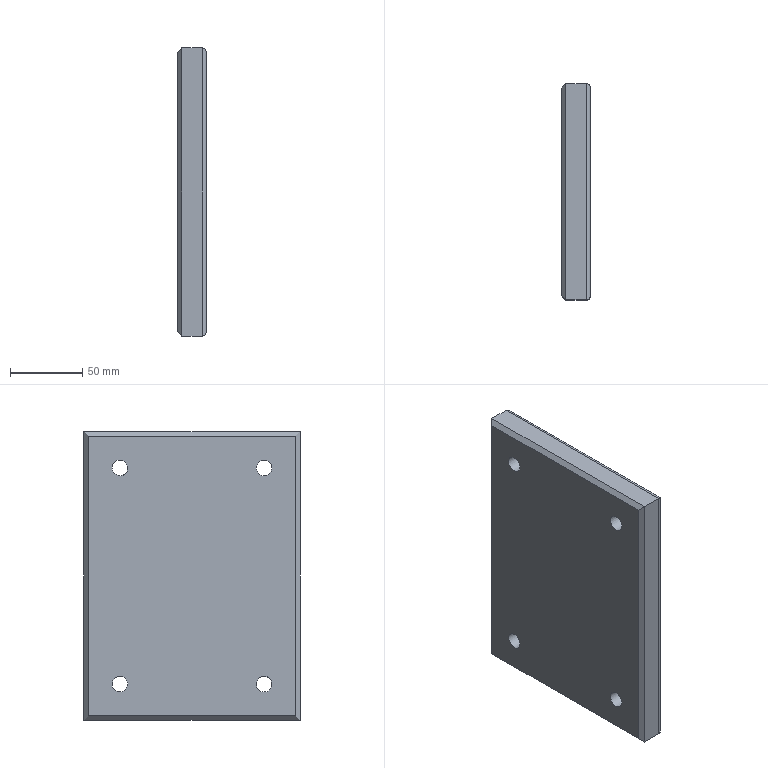Part | NX | features MAIN_BODY 2 | 1 solid | 30 faces | box 20 x 150 x 200 mm | volume 580501 mm3 | plane 14 | cylinder 12 | torus 4 | commonest cylinder face diameters 6 x4 11 x4 17.5 x4
STEP:
#1=CARTESIAN_POINT('',(910.,113.,-257.));
#2=VERTEX_POINT('',#1);
#3=CARTESIAN_POINT('',(910.,113.,-63.));
#4=VERTEX_POINT('',#3);
#5=CARTESIAN_POINT('',(910.,113.,-60.));
#6=DIRECTION('',(0.,0.,-1.));
#7=VECTOR('',#6,1000.);
#8=LINE('',#5,#7);
#9=EDGE_CURVE('',#2,#4,#8,.F.);
#10=ORIENTED_EDGE('',*,*,#9,.F.);
#11=CARTESIAN_POINT('',(910.,257.,-257.));
#12=VERTEX_POINT('',#11);
#13=CARTESIAN_POINT('',(910.,110.,-257.));
#14=DIRECTION('',(0.,1.,0.));
#15=VECTOR('',#14,1000.);
#16=LINE('',#13,#15);
#17=EDGE_CURVE('',#12,#2,#16,.F.);
#18=ORIENTED_EDGE('',*,*,#17,.F.);
#19=CARTESIAN_POINT('',(910.,257.,-63.));
#20=VERTEX_POINT('',#19);
#21=CARTESIAN_POINT('',(910.,257.,-260.));
#22=DIRECTION('',(0.,0.,1.));
#23=VECTOR('',#22,1000.);
#24=LINE('',#21,#23);
#25=EDGE_CURVE('',#20,#12,#24,.F.);
#26=ORIENTED_EDGE('',*,*,#25,.F.);
#27=CARTESIAN_POINT('',(910.,260.,-63.));
#28=DIRECTION('',(0.,-1.,0.));
#29=VECTOR('',#28,1000.);
#30=LINE('',#27,#29);
#31=EDGE_CURVE('',#4,#20,#30,.F.);
#32=ORIENTED_EDGE('',*,*,#31,.F.);
#33=EDGE_LOOP('',(#10,#18,#26,#32));
#34=FACE_BOUND('',#33,.T.);
#35=CARTESIAN_POINT('',(910.,135.,-96.75));
#36=VERTEX_POINT('',#35);
#37=CARTESIAN_POINT('',(910.,135.,-85.));
#38=DIRECTION('',(1.,0.,0.));
#39=DIRECTION('',(0.,0.,-1.));
#40=AXIS2_PLACEMENT_3D('',#37,#38,#39);
#41=CIRCLE('',#40,11.75);
#42=EDGE_CURVE('',#36,#36,#41,.T.);
#43=ORIENTED_EDGE('',*,*,#42,.F.);
#44=EDGE_LOOP('',(#43));
#45=FACE_BOUND('',#44,.T.);
#46=CARTESIAN_POINT('',(910.,235.,-96.75));
#47=VERTEX_POINT('',#46);
#48=CARTESIAN_POINT('',(910.,235.,-85.));
#49=DIRECTION('',(1.,0.,0.));
#50=DIRECTION('',(0.,0.,-1.));
#51=AXIS2_PLACEMENT_3D('',#48,#49,#50);
#52=CIRCLE('',#51,11.75);
#53=EDGE_CURVE('',#47,#47,#52,.T.);
#54=ORIENTED_EDGE('',*,*,#53,.F.);
#55=EDGE_LOOP('',(#54));
#56=FACE_BOUND('',#55,.T.);
#57=CARTESIAN_POINT('',(910.,235.,-246.75));
#58=VERTEX_POINT('',#57);
#59=CARTESIAN_POINT('',(910.,235.,-235.));
#60=DIRECTION('',(1.,0.,0.));
#61=DIRECTION('',(0.,0.,-1.));
#62=AXIS2_PLACEMENT_3D('',#59,#60,#61);
#63=CIRCLE('',#62,11.75);
#64=EDGE_CURVE('',#58,#58,#63,.T.);
#65=ORIENTED_EDGE('',*,*,#64,.F.);
#66=EDGE_LOOP('',(#65));
#67=FACE_BOUND('',#66,.T.);
#68=CARTESIAN_POINT('',(910.,135.,-246.75));
#69=VERTEX_POINT('',#68);
#70=CARTESIAN_POINT('',(910.,135.,-235.));
#71=DIRECTION('',(1.,0.,0.));
#72=DIRECTION('',(0.,0.,-1.));
#73=AXIS2_PLACEMENT_3D('',#70,#71,#72);
#74=CIRCLE('',#73,11.75);
#75=EDGE_CURVE('',#69,#69,#74,.T.);
#76=ORIENTED_EDGE('',*,*,#75,.F.);
#77=EDGE_LOOP('',(#76));
#78=FACE_BOUND('',#77,.T.);
#79=CARTESIAN_POINT('',(910.,110.,-260.));
#80=DIRECTION('',(-1.,0.,0.));
#81=DIRECTION('',(0.,0.,-1.));
#82=AXIS2_PLACEMENT_3D('',#79,#80,#81);
#83=PLANE('',#82);
#84=ADVANCED_FACE('',(#34,#45,#56,#67,#78),#83,.F.);
#85=CARTESIAN_POINT('',(890.,229.5,-235.));
#86=VERTEX_POINT('',#85);
#87=CARTESIAN_POINT('',(890.,235.,-235.));
#88=DIRECTION('',(-1.,0.,0.));
#89=DIRECTION('',(0.,-1.,0.));
#90=AXIS2_PLACEMENT_3D('',#87,#88,#89);
#91=CIRCLE('',#90,5.5);
#92=EDGE_CURVE('',#86,#86,#91,.T.);
#93=ORIENTED_EDGE('',*,*,#92,.T.);
#94=EDGE_LOOP('',(#93));
#95=FACE_BOUND('',#94,.T.);
#96=CARTESIAN_POINT('',(898.,235.,-229.5));
#97=VERTEX_POINT('',#96);
#98=CARTESIAN_POINT('',(898.,235.,-235.));
#99=DIRECTION('',(-1.,0.,0.));
#100=DIRECTION('',(0.,0.,1.));
#101=AXIS2_PLACEMENT_3D('',#98,#99,#100);
#102=CIRCLE('',#101,5.5);
#103=EDGE_CURVE('',#97,#97,#102,.T.);
#104=ORIENTED_EDGE('',*,*,#103,.F.);
#105=EDGE_LOOP('',(#104));
#106=FACE_BOUND('',#105,.T.);
#107=CARTESIAN_POINT('',(910.,235.,-235.));
#108=DIRECTION('',(-1.,0.,0.));
#109=DIRECTION('',(0.,0.,-1.));
#110=AXIS2_PLACEMENT_3D('',#107,#108,#109);
#111=CYLINDRICAL_SURFACE('',#110,5.5);
#112=ADVANCED_FACE('',(#95,#106),#111,.F.);
#113=CARTESIAN_POINT('',(890.,140.5,-85.));
#114=VERTEX_POINT('',#113);
#115=CARTESIAN_POINT('',(890.,135.,-85.));
#116=DIRECTION('',(-1.,0.,0.));
#117=DIRECTION('',(0.,1.,0.));
#118=AXIS2_PLACEMENT_3D('',#115,#116,#117);
#119=CIRCLE('',#118,5.5);
#120=EDGE_CURVE('',#114,#114,#119,.T.);
#121=ORIENTED_EDGE('',*,*,#120,.T.);
#122=EDGE_LOOP('',(#121));
#123=FACE_BOUND('',#122,.T.);
#124=CARTESIAN_POINT('',(898.,135.,-79.5));
#125=VERTEX_POINT('',#124);
#126=CARTESIAN_POINT('',(898.,135.,-85.));
#127=DIRECTION('',(-1.,0.,0.));
#128=DIRECTION('',(0.,0.,1.));
#129=AXIS2_PLACEMENT_3D('',#126,#127,#128);
#130=CIRCLE('',#129,5.5);
#131=EDGE_CURVE('',#125,#125,#130,.T.);
#132=ORIENTED_EDGE('',*,*,#131,.F.);
#133=EDGE_LOOP('',(#132));
#134=FACE_BOUND('',#133,.T.);
#135=CARTESIAN_POINT('',(910.,135.,-85.));
#136=DIRECTION('',(-1.,0.,0.));
#137=DIRECTION('',(0.,0.,-1.));
#138=AXIS2_PLACEMENT_3D('',#135,#136,#137);
#139=CYLINDRICAL_SURFACE('',#138,5.5);
#140=ADVANCED_FACE('',(#123,#134),#139,.F.);
#141=CARTESIAN_POINT('',(890.,257.,-257.));
#142=VERTEX_POINT('',#141);
#143=CARTESIAN_POINT('',(890.,257.,-63.));
#144=VERTEX_POINT('',#143);
#145=CARTESIAN_POINT('',(890.,257.,-260.));
#146=DIRECTION('',(0.,0.,1.));
#147=VECTOR('',#146,1000.);
#148=LINE('',#145,#147);
#149=EDGE_CURVE('',#142,#144,#148,.T.);
#150=ORIENTED_EDGE('',*,*,#149,.F.);
#151=CARTESIAN_POINT('',(890.,113.,-257.));
#152=VERTEX_POINT('',#151);
#153=CARTESIAN_POINT('',(890.,110.,-257.));
#154=DIRECTION('',(0.,1.,0.));
#155=VECTOR('',#154,1000.);
#156=LINE('',#153,#155);
#157=EDGE_CURVE('',#152,#142,#156,.T.);
#158=ORIENTED_EDGE('',*,*,#157,.F.);
#159=CARTESIAN_POINT('',(890.,113.,-63.));
#160=VERTEX_POINT('',#159);
#161=CARTESIAN_POINT('',(890.,113.,-260.));
#162=DIRECTION('',(0.,0.,-1.));
#163=VECTOR('',#162,1000.);
#164=LINE('',#161,#163);
#165=EDGE_CURVE('',#160,#152,#164,.T.);
#166=ORIENTED_EDGE('',*,*,#165,.F.);
#167=CARTESIAN_POINT('',(890.,110.,-63.));
#168=DIRECTION('',(0.,-1.,0.));
#169=VECTOR('',#168,1000.);
#170=LINE('',#167,#169);
#171=EDGE_CURVE('',#144,#160,#170,.T.);
#172=ORIENTED_EDGE('',*,*,#171,.F.);
#173=EDGE_LOOP('',(#150,#158,#166,#172));
#174=FACE_BOUND('',#173,.T.);
#175=CARTESIAN_POINT('',(890.,140.5,-235.));
#176=VERTEX_POINT('',#175);
#177=CARTESIAN_POINT('',(890.,135.,-235.));
#178=DIRECTION('',(1.,0.,0.));
#179=DIRECTION('',(0.,1.,0.));
#180=AXIS2_PLACEMENT_3D('',#177,#178,#179);
#181=CIRCLE('',#180,5.5);
#182=EDGE_CURVE('',#176,#176,#181,.T.);
#183=ORIENTED_EDGE('',*,*,#182,.T.);
#184=EDGE_LOOP('',(#183));
#185=FACE_BOUND('',#184,.T.);
#186=ORIENTED_EDGE('',*,*,#92,.F.);
#187=EDGE_LOOP('',(#186));
#188=FACE_BOUND('',#187,.T.);
#189=CARTESIAN_POINT('',(890.,229.5,-85.));
#190=VERTEX_POINT('',#189);
#191=CARTESIAN_POINT('',(890.,235.,-85.));
#192=DIRECTION('',(1.,0.,0.));
#193=DIRECTION('',(0.,-1.,0.));
#194=AXIS2_PLACEMENT_3D('',#191,#192,#193);
#195=CIRCLE('',#194,5.5);
#196=EDGE_CURVE('',#190,#190,#195,.T.);
#197=ORIENTED_EDGE('',*,*,#196,.T.);
#198=EDGE_LOOP('',(#197));
#199=FACE_BOUND('',#198,.T.);
#200=ORIENTED_EDGE('',*,*,#120,.F.);
#201=EDGE_LOOP('',(#200));
#202=FACE_BOUND('',#201,.T.);
#203=CARTESIAN_POINT('',(890.,110.,-260.));
#204=DIRECTION('',(-1.,0.,0.));
#205=DIRECTION('',(0.,0.,-1.));
#206=AXIS2_PLACEMENT_3D('',#203,#204,#205);
#207=PLANE('',#206);
#208=ADVANCED_FACE('',(#174,#185,#188,#199,#202),#207,.T.);
#209=CARTESIAN_POINT('',(907.,110.,-260.));
#210=VERTEX_POINT('',#209);
#211=CARTESIAN_POINT('',(893.,110.,-260.));
#212=VERTEX_POINT('',#211);
#213=CARTESIAN_POINT('',(910.,110.,-260.));
#214=DIRECTION('',(-1.,0.,0.));
#215=VECTOR('',#214,1000.);
#216=LINE('',#213,#215);
#217=EDGE_CURVE('',#210,#212,#216,.T.);
#218=ORIENTED_EDGE('',*,*,#217,.F.);
#219=CARTESIAN_POINT('',(907.,110.,-60.));
#220=VERTEX_POINT('',#219);
#221=CARTESIAN_POINT('',(907.,110.,-260.));
#222=DIRECTION('',(0.,0.,-1.));
#223=VECTOR('',#222,1000.);
#224=LINE('',#221,#223);
#225=EDGE_CURVE('',#220,#210,#224,.T.);
#226=ORIENTED_EDGE('',*,*,#225,.F.);
#227=CARTESIAN_POINT('',(893.,110.,-60.));
#228=VERTEX_POINT('',#227);
#229=CARTESIAN_POINT('',(910.,110.,-60.));
#230=DIRECTION('',(-1.,0.,0.));
#231=VECTOR('',#230,1000.);
#232=LINE('',#229,#231);
#233=EDGE_CURVE('',#220,#228,#232,.T.);
#234=ORIENTED_EDGE('',*,*,#233,.T.);
#235=CARTESIAN_POINT('',(893.,110.,-60.));
#236=DIRECTION('',(0.,0.,1.));
#237=VECTOR('',#236,1000.);
#238=LINE('',#235,#237);
#239=EDGE_CURVE('',#212,#228,#238,.T.);
#240=ORIENTED_EDGE('',*,*,#239,.F.);
#241=EDGE_LOOP('',(#218,#226,#234,#240));
#242=FACE_BOUND('',#241,.T.);
#243=CARTESIAN_POINT('',(910.,110.,-60.));
#244=DIRECTION('',(0.,-1.,0.));
#245=DIRECTION('',(0.,0.,1.));
#246=AXIS2_PLACEMENT_3D('',#243,#244,#245);
#247=PLANE('',#246);
#248=ADVANCED_FACE('',(#242),#247,.T.);
#249=CARTESIAN_POINT('',(907.,260.,-260.));
#250=VERTEX_POINT('',#249);
#251=CARTESIAN_POINT('',(893.,260.,-260.));
#252=VERTEX_POINT('',#251);
#253=CARTESIAN_POINT('',(910.,260.,-260.));
#254=DIRECTION('',(-1.,0.,0.));
#255=VECTOR('',#254,1000.);
#256=LINE('',#253,#255);
#257=EDGE_CURVE('',#250,#252,#256,.T.);
#258=ORIENTED_EDGE('',*,*,#257,.F.);
#259=CARTESIAN_POINT('',(907.,260.,-260.));
#260=DIRECTION('',(0.,1.,0.));
#261=VECTOR('',#260,1000.);
#262=LINE('',#259,#261);
#263=EDGE_CURVE('',#210,#250,#262,.T.);
#264=ORIENTED_EDGE('',*,*,#263,.F.);
#265=ORIENTED_EDGE('',*,*,#217,.T.);
#266=CARTESIAN_POINT('',(893.,110.,-260.));
#267=DIRECTION('',(0.,-1.,0.));
#268=VECTOR('',#267,1000.);
#269=LINE('',#266,#268);
#270=EDGE_CURVE('',#252,#212,#269,.T.);
#271=ORIENTED_EDGE('',*,*,#270,.F.);
#272=EDGE_LOOP('',(#258,#264,#265,#271));
#273=FACE_BOUND('',#272,.T.);
#274=CARTESIAN_POINT('',(910.,110.,-260.));
#275=DIRECTION('',(0.,0.,-1.));
#276=DIRECTION('',(0.,-1.,0.));
#277=AXIS2_PLACEMENT_3D('',#274,#275,#276);
#278=PLANE('',#277);
#279=ADVANCED_FACE('',(#273),#278,.T.);
#280=CARTESIAN_POINT('',(907.,260.,-60.));
#281=VERTEX_POINT('',#280);
#282=CARTESIAN_POINT('',(893.,260.,-60.));
#283=VERTEX_POINT('',#282);
#284=CARTESIAN_POINT('',(910.,260.,-60.));
#285=DIRECTION('',(-1.,0.,0.));
#286=VECTOR('',#285,1000.);
#287=LINE('',#284,#286);
#288=EDGE_CURVE('',#281,#283,#287,.T.);
#289=ORIENTED_EDGE('',*,*,#288,.F.);
#290=CARTESIAN_POINT('',(907.,260.,-60.));
#291=DIRECTION('',(0.,0.,1.));
#292=VECTOR('',#291,1000.);
#293=LINE('',#290,#292);
#294=EDGE_CURVE('',#250,#281,#293,.T.);
#295=ORIENTED_EDGE('',*,*,#294,.F.);
#296=ORIENTED_EDGE('',*,*,#257,.T.);
#297=CARTESIAN_POINT('',(893.,260.,-260.));
#298=DIRECTION('',(0.,0.,-1.));
#299=VECTOR('',#298,1000.);
#300=LINE('',#297,#299);
#301=EDGE_CURVE('',#283,#252,#300,.T.);
#302=ORIENTED_EDGE('',*,*,#301,.F.);
#303=EDGE_LOOP('',(#289,#295,#296,#302));
#304=FACE_BOUND('',#303,.T.);
#305=CARTESIAN_POINT('',(910.,260.,-260.));
#306=DIRECTION('',(0.,1.,0.));
#307=DIRECTION('',(0.,0.,-1.));
#308=AXIS2_PLACEMENT_3D('',#305,#306,#307);
#309=PLANE('',#308);
#310=ADVANCED_FACE('',(#304),#309,.T.);
#311=ORIENTED_EDGE('',*,*,#233,.F.);
#312=CARTESIAN_POINT('',(907.,110.,-60.));
#313=DIRECTION('',(0.,-1.,0.));
#314=VECTOR('',#313,1000.);
#315=LINE('',#312,#314);
#316=EDGE_CURVE('',#281,#220,#315,.T.);
#317=ORIENTED_EDGE('',*,*,#316,.F.);
#318=ORIENTED_EDGE('',*,*,#288,.T.);
#319=CARTESIAN_POINT('',(893.,260.,-60.));
#320=DIRECTION('',(0.,1.,0.));
#321=VECTOR('',#320,1000.);
#322=LINE('',#319,#321);
#323=EDGE_CURVE('',#228,#283,#322,.T.);
#324=ORIENTED_EDGE('',*,*,#323,.F.);
#325=EDGE_LOOP('',(#311,#317,#318,#324));
#326=FACE_BOUND('',#325,.T.);
#327=CARTESIAN_POINT('',(910.,260.,-60.));
#328=DIRECTION('',(0.,0.,1.));
#329=DIRECTION('',(0.,1.,0.));
#330=AXIS2_PLACEMENT_3D('',#327,#328,#329);
#331=PLANE('',#330);
#332=ADVANCED_FACE('',(#326),#331,.T.);
#333=CARTESIAN_POINT('',(898.,235.,-90.5));
#334=VERTEX_POINT('',#333);
#335=CARTESIAN_POINT('',(898.,235.,-85.));
#336=DIRECTION('',(1.,0.,0.));
#337=DIRECTION('',(0.,0.,-1.));
#338=AXIS2_PLACEMENT_3D('',#335,#336,#337);
#339=CIRCLE('',#338,5.5);
#340=EDGE_CURVE('',#334,#334,#339,.F.);
#341=ORIENTED_EDGE('',*,*,#340,.F.);
#342=EDGE_LOOP('',(#341));
#343=FACE_BOUND('',#342,.T.);
#344=ORIENTED_EDGE('',*,*,#196,.F.);
#345=EDGE_LOOP('',(#344));
#346=FACE_BOUND('',#345,.T.);
#347=CARTESIAN_POINT('',(910.,235.,-85.));
#348=DIRECTION('',(-1.,0.,0.));
#349=DIRECTION('',(0.,0.,-1.));
#350=AXIS2_PLACEMENT_3D('',#347,#348,#349);
#351=CYLINDRICAL_SURFACE('',#350,5.5);
#352=ADVANCED_FACE('',(#343,#346),#351,.F.);
#353=CARTESIAN_POINT('',(898.,135.,-240.5));
#354=VERTEX_POINT('',#353);
#355=CARTESIAN_POINT('',(898.,135.,-235.));
#356=DIRECTION('',(1.,0.,0.));
#357=DIRECTION('',(0.,0.,-1.));
#358=AXIS2_PLACEMENT_3D('',#355,#356,#357);
#359=CIRCLE('',#358,5.5);
#360=EDGE_CURVE('',#354,#354,#359,.F.);
#361=ORIENTED_EDGE('',*,*,#360,.F.);
#362=EDGE_LOOP('',(#361));
#363=FACE_BOUND('',#362,.T.);
#364=ORIENTED_EDGE('',*,*,#182,.F.);
#365=EDGE_LOOP('',(#364));
#366=FACE_BOUND('',#365,.T.);
#367=CARTESIAN_POINT('',(910.,135.,-235.));
#368=DIRECTION('',(-1.,0.,0.));
#369=DIRECTION('',(0.,0.,-1.));
#370=AXIS2_PLACEMENT_3D('',#367,#368,#369);
#371=CYLINDRICAL_SURFACE('',#370,5.5);
#372=ADVANCED_FACE('',(#363,#366),#371,.F.);
#373=CARTESIAN_POINT('',(907.,135.,-93.75));
#374=VERTEX_POINT('',#373);
#375=CARTESIAN_POINT('',(907.,135.,-85.));
#376=DIRECTION('',(1.,0.,0.));
#377=DIRECTION('',(0.,0.,-1.));
#378=AXIS2_PLACEMENT_3D('',#375,#376,#377);
#379=CIRCLE('',#378,8.75);
#380=EDGE_CURVE('',#374,#374,#379,.F.);
#381=ORIENTED_EDGE('',*,*,#380,.F.);
#382=EDGE_LOOP('',(#381));
#383=FACE_BOUND('',#382,.T.);
#384=CARTESIAN_POINT('',(898.,143.75,-85.));
#385=VERTEX_POINT('',#384);
#386=CARTESIAN_POINT('',(898.,135.,-85.));
#387=DIRECTION('',(-1.,0.,0.));
#388=DIRECTION('',(0.,1.,0.));
#389=AXIS2_PLACEMENT_3D('',#386,#387,#388);
#390=CIRCLE('',#389,8.75);
#391=EDGE_CURVE('',#385,#385,#390,.T.);
#392=ORIENTED_EDGE('',*,*,#391,.T.);
#393=EDGE_LOOP('',(#392));
#394=FACE_BOUND('',#393,.T.);
#395=CARTESIAN_POINT('',(920.,135.,-85.));
#396=DIRECTION('',(-1.,0.,0.));
#397=DIRECTION('',(0.,0.,-1.));
#398=AXIS2_PLACEMENT_3D('',#395,#396,#397);
#399=CYLINDRICAL_SURFACE('',#398,8.75);
#400=ADVANCED_FACE('',(#383,#394),#399,.F.);
#401=ORIENTED_EDGE('',*,*,#131,.T.);
#402=EDGE_LOOP('',(#401));
#403=FACE_BOUND('',#402,.T.);
#404=ORIENTED_EDGE('',*,*,#391,.F.);
#405=EDGE_LOOP('',(#404));
#406=FACE_BOUND('',#405,.T.);
#407=CARTESIAN_POINT('',(898.,135.,-85.));
#408=DIRECTION('',(1.,0.,0.));
#409=DIRECTION('',(0.,0.,1.));
#410=AXIS2_PLACEMENT_3D('',#407,#408,#409);
#411=PLANE('',#410);
#412=ADVANCED_FACE('',(#403,#406),#411,.T.);
#413=CARTESIAN_POINT('',(907.,135.,-243.75));
#414=VERTEX_POINT('',#413);
#415=CARTESIAN_POINT('',(907.,135.,-235.));
#416=DIRECTION('',(1.,0.,0.));
#417=DIRECTION('',(0.,0.,-1.));
#418=AXIS2_PLACEMENT_3D('',#415,#416,#417);
#419=CIRCLE('',#418,8.75);
#420=EDGE_CURVE('',#414,#414,#419,.F.);
#421=ORIENTED_EDGE('',*,*,#420,.F.);
#422=EDGE_LOOP('',(#421));
#423=FACE_BOUND('',#422,.T.);
#424=CARTESIAN_POINT('',(898.,143.75,-235.));
#425=VERTEX_POINT('',#424);
#426=CARTESIAN_POINT('',(898.,135.,-235.));
#427=DIRECTION('',(1.,0.,0.));
#428=DIRECTION('',(0.,1.,0.));
#429=AXIS2_PLACEMENT_3D('',#426,#427,#428);
#430=CIRCLE('',#429,8.75);
#431=EDGE_CURVE('',#425,#425,#430,.T.);
#432=ORIENTED_EDGE('',*,*,#431,.F.);
#433=EDGE_LOOP('',(#432));
#434=FACE_BOUND('',#433,.T.);
#435=CARTESIAN_POINT('',(920.,135.,-235.));
#436=DIRECTION('',(-1.,0.,0.));
#437=DIRECTION('',(0.,0.,-1.));
#438=AXIS2_PLACEMENT_3D('',#435,#436,#437);
#439=CYLINDRICAL_SURFACE('',#438,8.75);
#440=ADVANCED_FACE('',(#423,#434),#439,.F.);
#441=ORIENTED_EDGE('',*,*,#431,.T.);
#442=EDGE_LOOP('',(#441));
#443=FACE_BOUND('',#442,.T.);
#444=ORIENTED_EDGE('',*,*,#360,.T.);
#445=EDGE_LOOP('',(#444));
#446=FACE_BOUND('',#445,.T.);
#447=CARTESIAN_POINT('',(898.,135.,-235.));
#448=DIRECTION('',(-1.,0.,0.));
#449=DIRECTION('',(0.,0.,-1.));
#450=AXIS2_PLACEMENT_3D('',#447,#448,#449);
#451=PLANE('',#450);
#452=ADVANCED_FACE('',(#443,#446),#451,.F.);
#453=CARTESIAN_POINT('',(907.,235.,-93.75));
#454=VERTEX_POINT('',#453);
#455=CARTESIAN_POINT('',(907.,235.,-85.));
#456=DIRECTION('',(1.,0.,0.));
#457=DIRECTION('',(0.,0.,-1.));
#458=AXIS2_PLACEMENT_3D('',#455,#456,#457);
#459=CIRCLE('',#458,8.75);
#460=EDGE_CURVE('',#454,#454,#459,.F.);
#461=ORIENTED_EDGE('',*,*,#460,.F.);
#462=EDGE_LOOP('',(#461));
#463=FACE_BOUND('',#462,.T.);
#464=CARTESIAN_POINT('',(898.,226.25,-85.));
#465=VERTEX_POINT('',#464);
#466=CARTESIAN_POINT('',(898.,235.,-85.));
#467=DIRECTION('',(1.,0.,0.));
#468=DIRECTION('',(0.,-1.,0.));
#469=AXIS2_PLACEMENT_3D('',#466,#467,#468);
#470=CIRCLE('',#469,8.75);
#471=EDGE_CURVE('',#465,#465,#470,.T.);
#472=ORIENTED_EDGE('',*,*,#471,.F.);
#473=EDGE_LOOP('',(#472));
#474=FACE_BOUND('',#473,.T.);
#475=CARTESIAN_POINT('',(920.,235.,-85.));
#476=DIRECTION('',(-1.,0.,0.));
#477=DIRECTION('',(0.,0.,-1.));
#478=AXIS2_PLACEMENT_3D('',#475,#476,#477);
#479=CYLINDRICAL_SURFACE('',#478,8.75);
#480=ADVANCED_FACE('',(#463,#474),#479,.F.);
#481=ORIENTED_EDGE('',*,*,#471,.T.);
#482=EDGE_LOOP('',(#481));
#483=FACE_BOUND('',#482,.T.);
#484=ORIENTED_EDGE('',*,*,#340,.T.);
#485=EDGE_LOOP('',(#484));
#486=FACE_BOUND('',#485,.T.);
#487=CARTESIAN_POINT('',(898.,235.,-85.));
#488=DIRECTION('',(-1.,0.,0.));
#489=DIRECTION('',(0.,0.,-1.));
#490=AXIS2_PLACEMENT_3D('',#487,#488,#489);
#491=PLANE('',#490);
#492=ADVANCED_FACE('',(#483,#486),#491,.F.);
#493=CARTESIAN_POINT('',(907.,235.,-243.75));
#494=VERTEX_POINT('',#493);
#495=CARTESIAN_POINT('',(907.,235.,-235.));
#496=DIRECTION('',(1.,0.,0.));
#497=DIRECTION('',(0.,0.,-1.));
#498=AXIS2_PLACEMENT_3D('',#495,#496,#497);
#499=CIRCLE('',#498,8.75);
#500=EDGE_CURVE('',#494,#494,#499,.F.);
#501=ORIENTED_EDGE('',*,*,#500,.F.);
#502=EDGE_LOOP('',(#501));
#503=FACE_BOUND('',#502,.T.);
#504=CARTESIAN_POINT('',(898.,226.25,-235.));
#505=VERTEX_POINT('',#504);
#506=CARTESIAN_POINT('',(898.,235.,-235.));
#507=DIRECTION('',(-1.,0.,0.));
#508=DIRECTION('',(0.,-1.,0.));
#509=AXIS2_PLACEMENT_3D('',#506,#507,#508);
#510=CIRCLE('',#509,8.75);
#511=EDGE_CURVE('',#505,#505,#510,.T.);
#512=ORIENTED_EDGE('',*,*,#511,.T.);
#513=EDGE_LOOP('',(#512));
#514=FACE_BOUND('',#513,.T.);
#515=CARTESIAN_POINT('',(920.,235.,-235.));
#516=DIRECTION('',(-1.,0.,0.));
#517=DIRECTION('',(0.,0.,-1.));
#518=AXIS2_PLACEMENT_3D('',#515,#516,#517);
#519=CYLINDRICAL_SURFACE('',#518,8.75);
#520=ADVANCED_FACE('',(#503,#514),#519,.F.);
#521=ORIENTED_EDGE('',*,*,#103,.T.);
#522=EDGE_LOOP('',(#521));
#523=FACE_BOUND('',#522,.T.);
#524=ORIENTED_EDGE('',*,*,#511,.F.);
#525=EDGE_LOOP('',(#524));
#526=FACE_BOUND('',#525,.T.);
#527=CARTESIAN_POINT('',(898.,235.,-235.));
#528=DIRECTION('',(1.,0.,0.));
#529=DIRECTION('',(0.,0.,1.));
#530=AXIS2_PLACEMENT_3D('',#527,#528,#529);
#531=PLANE('',#530);
#532=ADVANCED_FACE('',(#523,#526),#531,.T.);
#533=CARTESIAN_POINT('',(907.,113.,-257.));
#534=DIRECTION('',(0.,0.7071,-0.7071));
#535=DIRECTION('',(0.,-0.7071,-0.7071));
#536=AXIS2_PLACEMENT_3D('',#533,#534,#535);
#537=ELLIPSE('',#536,4.243,3.);
#538=EDGE_CURVE('',#2,#210,#537,.T.);
#539=ORIENTED_EDGE('',*,*,#538,.T.);
#540=ORIENTED_EDGE('',*,*,#263,.T.);
#541=CARTESIAN_POINT('',(907.,257.,-257.));
#542=DIRECTION('',(0.,0.7071,0.7071));
#543=DIRECTION('',(0.,-0.7071,0.7071));
#544=AXIS2_PLACEMENT_3D('',#541,#542,#543);
#545=ELLIPSE('',#544,4.243,3.);
#546=EDGE_CURVE('',#250,#12,#545,.F.);
#547=ORIENTED_EDGE('',*,*,#546,.T.);
#548=ORIENTED_EDGE('',*,*,#17,.T.);
#549=EDGE_LOOP('',(#539,#540,#547,#548));
#550=FACE_BOUND('',#549,.T.);
#551=CARTESIAN_POINT('',(907.,110.,-257.));
#552=DIRECTION('',(0.,-1.,0.));
#553=DIRECTION('',(0.,0.,1.));
#554=AXIS2_PLACEMENT_3D('',#551,#552,#553);
#555=CYLINDRICAL_SURFACE('',#554,3.);
#556=ADVANCED_FACE('',(#550),#555,.T.);
#557=ORIENTED_EDGE('',*,*,#546,.F.);
#558=ORIENTED_EDGE('',*,*,#294,.T.);
#559=CARTESIAN_POINT('',(907.,257.,-63.));
#560=DIRECTION('',(0.,-0.7071,0.7071));
#561=DIRECTION('',(0.,-0.7071,-0.7071));
#562=AXIS2_PLACEMENT_3D('',#559,#560,#561);
#563=ELLIPSE('',#562,4.243,3.);
#564=EDGE_CURVE('',#281,#20,#563,.F.);
#565=ORIENTED_EDGE('',*,*,#564,.T.);
#566=ORIENTED_EDGE('',*,*,#25,.T.);
#567=EDGE_LOOP('',(#557,#558,#565,#566));
#568=FACE_BOUND('',#567,.T.);
#569=CARTESIAN_POINT('',(907.,257.,-260.));
#570=DIRECTION('',(0.,0.,-1.));
#571=DIRECTION('',(1.,0.,0.));
#572=AXIS2_PLACEMENT_3D('',#569,#570,#571);
#573=CYLINDRICAL_SURFACE('',#572,3.);
#574=ADVANCED_FACE('',(#568),#573,.T.);
#575=ORIENTED_EDGE('',*,*,#538,.F.);
#576=ORIENTED_EDGE('',*,*,#9,.T.);
#577=CARTESIAN_POINT('',(907.,113.,-63.));
#578=DIRECTION('',(0.,-0.7071,-0.7071));
#579=DIRECTION('',(0.,-0.7071,0.7071));
#580=AXIS2_PLACEMENT_3D('',#577,#578,#579);
#581=ELLIPSE('',#580,4.243,3.);
#582=EDGE_CURVE('',#4,#220,#581,.T.);
#583=ORIENTED_EDGE('',*,*,#582,.T.);
#584=ORIENTED_EDGE('',*,*,#225,.T.);
#585=EDGE_LOOP('',(#575,#576,#583,#584));
#586=FACE_BOUND('',#585,.T.);
#587=CARTESIAN_POINT('',(907.,113.,-60.));
#588=DIRECTION('',(0.,0.,1.));
#589=DIRECTION('',(0.,1.,0.));
#590=AXIS2_PLACEMENT_3D('',#587,#588,#589);
#591=CYLINDRICAL_SURFACE('',#590,3.);
#592=ADVANCED_FACE('',(#586),#591,.T.);
#593=ORIENTED_EDGE('',*,*,#564,.F.);
#594=ORIENTED_EDGE('',*,*,#316,.T.);
#595=ORIENTED_EDGE('',*,*,#582,.F.);
#596=ORIENTED_EDGE('',*,*,#31,.T.);
#597=EDGE_LOOP('',(#593,#594,#595,#596));
#598=FACE_BOUND('',#597,.T.);
#599=CARTESIAN_POINT('',(907.,260.,-63.));
#600=DIRECTION('',(0.,1.,0.));
#601=DIRECTION('',(0.,0.,-1.));
#602=AXIS2_PLACEMENT_3D('',#599,#600,#601);
#603=CYLINDRICAL_SURFACE('',#602,3.);
#604=ADVANCED_FACE('',(#598),#603,.T.);
#605=ORIENTED_EDGE('',*,*,#42,.T.);
#606=EDGE_LOOP('',(#605));
#607=FACE_BOUND('',#606,.T.);
#608=ORIENTED_EDGE('',*,*,#380,.T.);
#609=EDGE_LOOP('',(#608));
#610=FACE_BOUND('',#609,.T.);
#611=CARTESIAN_POINT('',(907.,135.,-85.));
#612=DIRECTION('',(-1.,0.,0.));
#613=DIRECTION('',(0.,0.,-1.));
#614=AXIS2_PLACEMENT_3D('',#611,#612,#613);
#615=TOROIDAL_SURFACE('',#614,11.75,3.);
#616=ADVANCED_FACE('',(#607,#610),#615,.T.);
#617=ORIENTED_EDGE('',*,*,#460,.T.);
#618=EDGE_LOOP('',(#617));
#619=FACE_BOUND('',#618,.T.);
#620=ORIENTED_EDGE('',*,*,#53,.T.);
#621=EDGE_LOOP('',(#620));
#622=FACE_BOUND('',#621,.T.);
#623=CARTESIAN_POINT('',(907.,235.,-85.));
#624=DIRECTION('',(-1.,0.,0.));
#625=DIRECTION('',(0.,0.,-1.));
#626=AXIS2_PLACEMENT_3D('',#623,#624,#625);
#627=TOROIDAL_SURFACE('',#626,11.75,3.);
#628=ADVANCED_FACE('',(#619,#622),#627,.T.);
#629=ORIENTED_EDGE('',*,*,#64,.T.);
#630=EDGE_LOOP('',(#629));
#631=FACE_BOUND('',#630,.T.);
#632=ORIENTED_EDGE('',*,*,#500,.T.);
#633=EDGE_LOOP('',(#632));
#634=FACE_BOUND('',#633,.T.);
#635=CARTESIAN_POINT('',(907.,235.,-235.));
#636=DIRECTION('',(-1.,0.,0.));
#637=DIRECTION('',(0.,0.,-1.));
#638=AXIS2_PLACEMENT_3D('',#635,#636,#637);
#639=TOROIDAL_SURFACE('',#638,11.75,3.);
#640=ADVANCED_FACE('',(#631,#634),#639,.T.);
#641=ORIENTED_EDGE('',*,*,#420,.T.);
#642=EDGE_LOOP('',(#641));
#643=FACE_BOUND('',#642,.T.);
#644=ORIENTED_EDGE('',*,*,#75,.T.);
#645=EDGE_LOOP('',(#644));
#646=FACE_BOUND('',#645,.T.);
#647=CARTESIAN_POINT('',(907.,135.,-235.));
#648=DIRECTION('',(-1.,0.,0.));
#649=DIRECTION('',(0.,0.,-1.));
#650=AXIS2_PLACEMENT_3D('',#647,#648,#649);
#651=TOROIDAL_SURFACE('',#650,11.75,3.);
#652=ADVANCED_FACE('',(#643,#646),#651,.T.);
#653=CARTESIAN_POINT('',(891.,112.,-258.));
#654=DIRECTION('',(0.5774,-0.5774,-0.5774));
#655=VECTOR('',#654,1000.);
#656=LINE('',#653,#655);
#657=EDGE_CURVE('',#212,#152,#656,.F.);
#658=ORIENTED_EDGE('',*,*,#657,.T.);
#659=ORIENTED_EDGE('',*,*,#157,.T.);
#660=CARTESIAN_POINT('',(891.,258.,-258.));
#661=DIRECTION('',(0.5774,0.5774,-0.5774));
#662=VECTOR('',#661,1000.);
#663=LINE('',#660,#662);
#664=EDGE_CURVE('',#142,#252,#663,.T.);
#665=ORIENTED_EDGE('',*,*,#664,.T.);
#666=ORIENTED_EDGE('',*,*,#270,.T.);
#667=EDGE_LOOP('',(#658,#659,#665,#666));
#668=FACE_BOUND('',#667,.T.);
#669=CARTESIAN_POINT('',(890.,110.,-257.));
#670=DIRECTION('',(0.7071,0.,0.7071));
#671=DIRECTION('',(-0.7071,0.,0.7071));
#672=AXIS2_PLACEMENT_3D('',#669,#670,#671);
#673=PLANE('',#672);
#674=ADVANCED_FACE('',(#668),#673,.F.);
#675=ORIENTED_EDGE('',*,*,#664,.F.);
#676=ORIENTED_EDGE('',*,*,#149,.T.);
#677=CARTESIAN_POINT('',(824.333,191.333,-128.667));
#678=DIRECTION('',(-0.5774,-0.5774,-0.5774));
#679=VECTOR('',#678,1000.);
#680=LINE('',#677,#679);
#681=EDGE_CURVE('',#144,#283,#680,.F.);
#682=ORIENTED_EDGE('',*,*,#681,.T.);
#683=ORIENTED_EDGE('',*,*,#301,.T.);
#684=EDGE_LOOP('',(#675,#676,#682,#683));
#685=FACE_BOUND('',#684,.T.);
#686=CARTESIAN_POINT('',(890.,257.,-260.));
#687=DIRECTION('',(0.7071,-0.7071,0.));
#688=DIRECTION('',(0.7071,0.7071,0.));
#689=AXIS2_PLACEMENT_3D('',#686,#687,#688);
#690=PLANE('',#689);
#691=ADVANCED_FACE('',(#685),#690,.F.);
#692=ORIENTED_EDGE('',*,*,#657,.F.);
#693=ORIENTED_EDGE('',*,*,#239,.T.);
#694=CARTESIAN_POINT('',(824.333,178.667,-128.667));
#695=DIRECTION('',(0.5774,-0.5774,0.5774));
#696=VECTOR('',#695,1000.);
#697=LINE('',#694,#696);
#698=EDGE_CURVE('',#228,#160,#697,.F.);
#699=ORIENTED_EDGE('',*,*,#698,.T.);
#700=ORIENTED_EDGE('',*,*,#165,.T.);
#701=EDGE_LOOP('',(#692,#693,#699,#700));
#702=FACE_BOUND('',#701,.T.);
#703=CARTESIAN_POINT('',(890.,113.,-260.));
#704=DIRECTION('',(0.7071,0.7071,0.));
#705=DIRECTION('',(-0.7071,0.7071,0.));
#706=AXIS2_PLACEMENT_3D('',#703,#704,#705);
#707=PLANE('',#706);
#708=ADVANCED_FACE('',(#702),#707,.F.);
#709=ORIENTED_EDGE('',*,*,#681,.F.);
#710=ORIENTED_EDGE('',*,*,#171,.T.);
#711=ORIENTED_EDGE('',*,*,#698,.F.);
#712=ORIENTED_EDGE('',*,*,#323,.T.);
#713=EDGE_LOOP('',(#709,#710,#711,#712));
#714=FACE_BOUND('',#713,.T.);
#715=CARTESIAN_POINT('',(890.,110.,-63.));
#716=DIRECTION('',(0.7071,0.,-0.7071));
#717=DIRECTION('',(0.7071,0.,0.7071));
#718=AXIS2_PLACEMENT_3D('',#715,#716,#717);
#719=PLANE('',#718);
#720=ADVANCED_FACE('',(#714),#719,.F.);
#721=CLOSED_SHELL('',(#84,#112,#140,#208,#248,#279,#310,#332,#352,#372,#400,#412,#440,#452,#480,#492,#520,#532,#556,#574,#592,#604,#616,#628,#640,#652,#674,#691,#708,#720));
#722=MANIFOLD_SOLID_BREP('',#721);
#723=(LENGTH_UNIT()NAMED_UNIT(*)SI_UNIT(.MILLI.,.METRE.));
#724=UNCERTAINTY_MEASURE_WITH_UNIT(LENGTH_MEASURE(0.00001),#723,'','');
#725=(NAMED_UNIT(*)PLANE_ANGLE_UNIT()SI_UNIT($,.RADIAN.));
#726=(NAMED_UNIT(*)SI_UNIT($,.STERADIAN.)SOLID_ANGLE_UNIT());
#727=(GEOMETRIC_REPRESENTATION_CONTEXT(3)GLOBAL_UNCERTAINTY_ASSIGNED_CONTEXT((#724))GLOBAL_UNIT_ASSIGNED_CONTEXT((#723,#725,#726))REPRESENTATION_CONTEXT('',''));
#728=ADVANCED_BREP_SHAPE_REPRESENTATION('',(#722),#727);